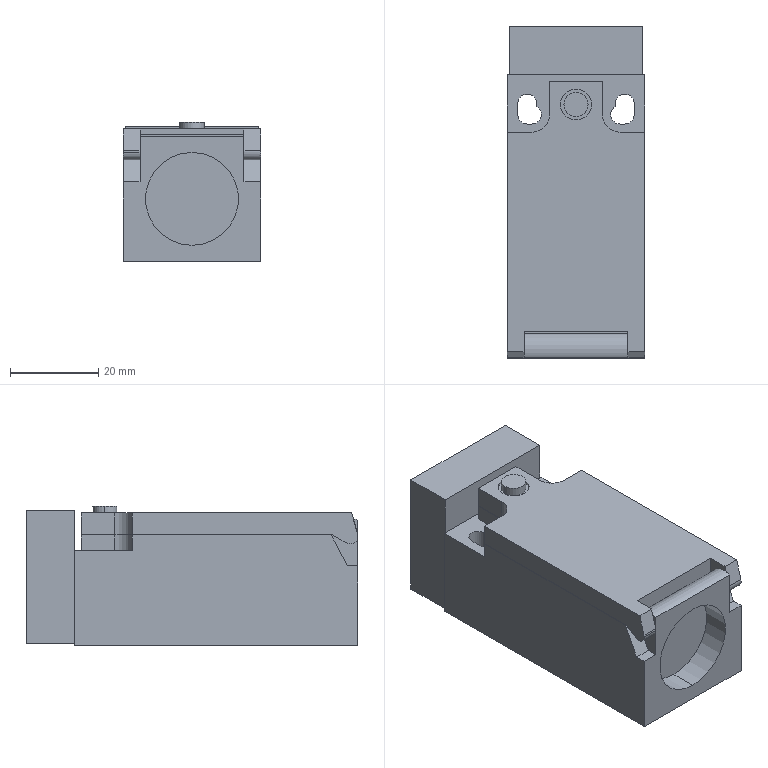Part | STEP file | D4NS_1CF_BASE^D4NS_1CF_Laser guard | 1 solid | 119 faces | box 31 x 75 x 31.5 mm | volume 57393 mm3 | plane 80 | cylinder 39 | commonest cylinder face diameters 3 x8 4.3 x7 8 x5 4 x4 6 x4 3.5 x3